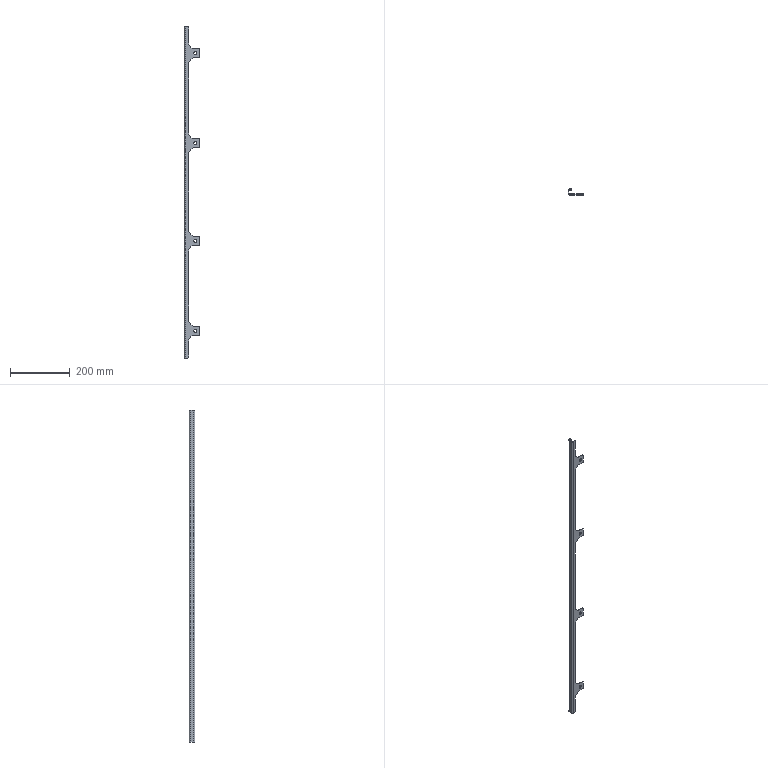Part | STEP file | 750078185 | 1 solid | 58 faces | box 52 x 20 x 1107 mm | volume 119219 mm3 | cylinder 32 | plane 26 | commonest cylinder face diameters 6 x12 10.5 x8 40 x8 5 x2 10 x2